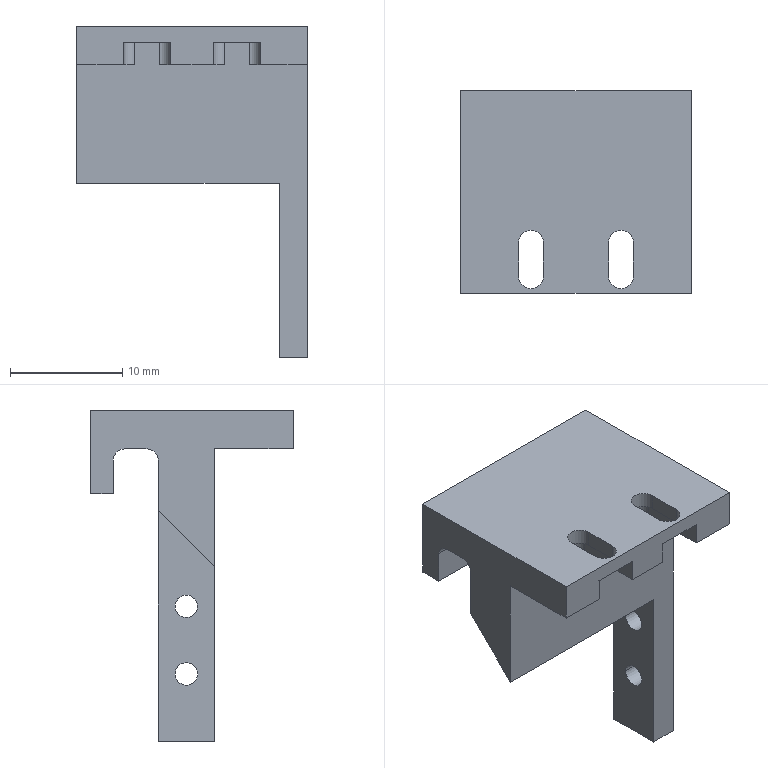CAM job | NX | 3-axis milling | part box 20.5 x 18 x 29.4 mm | stock box 24.5 x 22 x 30.4 mm
Tools:
number,name,description,diameter,corner_radius,flute_length,length,flutes
9,D10JING,Milling Tool-5 Parameters,10.0,0.0,50.0,75.0,2
10,D10,Milling Tool-5 Parameters,10.0,0.0,50.0,75.0,2
2,D2,Milling Tool-5 Parameters,2.0,0.0,50.0,75.0,2
5,D2R0.5,Milling Tool-5 Parameters,2.0,0.5,50.0,75.0,2
8,R1,Milling Tool-5 Parameters,2.0,1.0,50.0,75.0,2
7,D4A45,Milling Tool-5 Parameters,4.0,0.0,50.0,75.0,2
Operations:
program,operation,operation_type,tool,method,geometry_group,spindle_rpm,surface_speed,feed_per_tooth,feed_cut,feed_plunge,cut_length_mm,path_length_mm,cut_time_min,machine_time_min
1,FLOOR_WALL,VolumeBased25DMillingOperation,D10JING,METHOD,A,9500.0,298.0,0.0658,1250.0,100.0,202.497,256.497,0.162,0.1674
1,ZLEVEL_PROFILE,ZLevelMilling,D10,METHOD,A,9500.0,298.0,0.1316,2500.0,1000.0,6501.788,6588.038,2.624,2.632
1,CAVITY_MILL,CavityMilling,D10,METHOD,A,9500.0,298.0,0.1579,3000.0,1000.0,9560.393,10477.098,3.888,3.98
1,11,ZLevelMilling,D10JING,METHOD,A,9500.0,298.0,0.0632,1200.0,1000.0,543.269,1150.776,0.4574,0.5181
1,CAVITY_MILL_COPY_COPY,CavityMilling,D2,METHOD,A,7500.0,70.0,0.0567,850.0,1000.0,7203.216,8087.658,8.248,8.337
1,ZLEVEL_PROFILE_1,ZLevelMilling,D2R0.5,METHOD,A,9500.0,89.0,0.1316,2500.0,1000.0,1720.303,1810.814,0.6903,0.6994
1,ZLEVEL_PROFILE_1_COPY,ZLevelMilling,R1,METHOD,A,9500.0,89.0,0.1316,2500.0,1000.0,334.923,930.723,0.1445,0.2041
1,PLANAR_MILL_COPY_1,PlanarMilling,D4A45,METHOD,A,9500.0,179.0,0.0658,1250.0,100.0,25.992,84.992,0.0208,0.0267
1,PLANAR_MILL_COPY_1_COPY,PlanarMilling,D4A45,METHOD,A,9500.0,179.0,0.0658,1250.0,100.0,55.992,158.992,0.0448,0.0551
1,PLANAR_MILL_COPY_1_COPY_COPY,PlanarMilling,D4A45,METHOD,A,9500.0,179.0,0.0658,1250.0,100.0,61.816,172.815,0.0495,0.0606